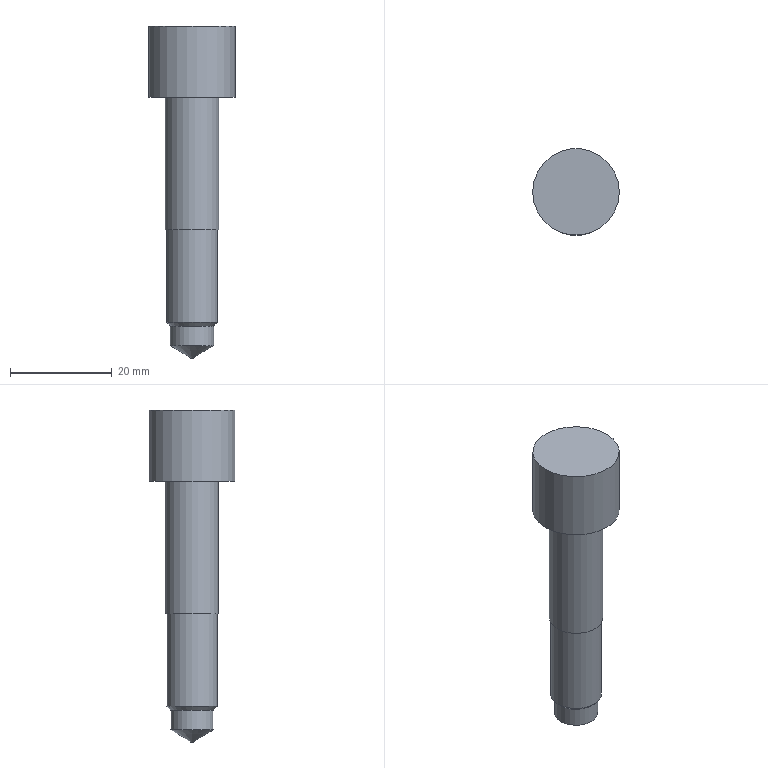Part | NX | features BREP 2 | 2 solids | 21 faces | box 17 x 17 x 65.231 mm | volume 11942 mm3 | plane 14 | cylinder 5 | cone 2 | commonest cylinder face diameters 8.5 x1 10 x1 10.5 x1 16 x1 17 x1
STEP:
#1=CARTESIAN_POINT('',(-4.25,0.,-40.));
#2=VERTEX_POINT('',#1);
#3=CARTESIAN_POINT('',(0.,0.,-40.));
#4=DIRECTION('',(0.,0.,1.));
#5=DIRECTION('',(-1.,0.,0.));
#6=AXIS2_PLACEMENT_3D('',#3,#4,#5);
#7=CIRCLE('',#6,4.25);
#8=EDGE_CURVE('',#2,#2,#7,.T.);
#9=ORIENTED_EDGE('',*,*,#8,.F.);
#10=EDGE_LOOP('',(#9));
#11=FACE_BOUND('',#10,.T.);
#12=CARTESIAN_POINT('',(-4.25,0.,-62.8));
#13=VERTEX_POINT('',#12);
#14=CARTESIAN_POINT('',(0.,0.,-62.8));
#15=DIRECTION('',(0.,0.,-1.));
#16=DIRECTION('',(-1.,0.,0.));
#17=AXIS2_PLACEMENT_3D('',#14,#15,#16);
#18=CIRCLE('',#17,4.25);
#19=EDGE_CURVE('',#13,#13,#18,.T.);
#20=ORIENTED_EDGE('',*,*,#19,.F.);
#21=EDGE_LOOP('',(#20));
#22=FACE_BOUND('',#21,.T.);
#23=CARTESIAN_POINT('',(0.,0.,-62.8));
#24=DIRECTION('',(0.,0.,1.));
#25=DIRECTION('',(-1.,0.,0.));
#26=AXIS2_PLACEMENT_3D('',#23,#24,#25);
#27=CYLINDRICAL_SURFACE('',#26,4.25);
#28=ADVANCED_FACE('',(#11,#22),#27,.T.);
#29=CARTESIAN_POINT('',(-0.2034,0.,-65.231));
#30=VERTEX_POINT('',#29);
#31=CARTESIAN_POINT('',(0.,0.,-65.231));
#32=DIRECTION('',(0.,0.,-1.));
#33=DIRECTION('',(-1.,0.,0.));
#34=AXIS2_PLACEMENT_3D('',#31,#32,#33);
#35=CIRCLE('',#34,0.2034);
#36=EDGE_CURVE('',#30,#30,#35,.T.);
#37=ORIENTED_EDGE('',*,*,#36,.T.);
#38=EDGE_LOOP('',(#37));
#39=FACE_BOUND('',#38,.T.);
#40=CARTESIAN_POINT('',(0.,0.,-65.231));
#41=DIRECTION('',(0.,0.,-1.));
#42=DIRECTION('',(1.,0.,0.));
#43=AXIS2_PLACEMENT_3D('',#40,#41,#42);
#44=PLANE('',#43);
#45=ADVANCED_FACE('',(#39),#44,.T.);
#46=ORIENTED_EDGE('',*,*,#36,.F.);
#47=EDGE_LOOP('',(#46));
#48=FACE_BOUND('',#47,.T.);
#49=ORIENTED_EDGE('',*,*,#19,.T.);
#50=EDGE_LOOP('',(#49));
#51=FACE_BOUND('',#50,.T.);
#52=CARTESIAN_POINT('',(0.,0.,-62.8));
#53=DIRECTION('',(0.,0.,1.));
#54=DIRECTION('',(-1.,0.,0.));
#55=AXIS2_PLACEMENT_3D('',#52,#53,#54);
#56=CONICAL_SURFACE('',#55,4.25,1.03);
#57=ADVANCED_FACE('',(#48,#51),#56,.T.);
#58=ORIENTED_EDGE('',*,*,#8,.T.);
#59=EDGE_LOOP('',(#58));
#60=FACE_BOUND('',#59,.T.);
#61=CARTESIAN_POINT('',(-5.25,0.,-40.));
#62=VERTEX_POINT('',#61);
#63=CARTESIAN_POINT('',(0.,0.,-40.));
#64=DIRECTION('',(0.,0.,-1.));
#65=DIRECTION('',(-1.,0.,0.));
#66=AXIS2_PLACEMENT_3D('',#63,#64,#65);
#67=CIRCLE('',#66,5.25);
#68=EDGE_CURVE('',#62,#62,#67,.T.);
#69=ORIENTED_EDGE('',*,*,#68,.T.);
#70=EDGE_LOOP('',(#69));
#71=FACE_BOUND('',#70,.T.);
#72=CARTESIAN_POINT('',(0.,0.,-40.));
#73=DIRECTION('',(0.,0.,-1.));
#74=DIRECTION('',(1.,0.,0.));
#75=AXIS2_PLACEMENT_3D('',#72,#73,#74);
#76=PLANE('',#75);
#77=ADVANCED_FACE('',(#60,#71),#76,.T.);
#78=ORIENTED_EDGE('',*,*,#68,.F.);
#79=EDGE_LOOP('',(#78));
#80=FACE_BOUND('',#79,.T.);
#81=CARTESIAN_POINT('',(-5.25,0.,-14.));
#82=VERTEX_POINT('',#81);
#83=CARTESIAN_POINT('',(0.,0.,-14.));
#84=DIRECTION('',(0.,0.,-1.));
#85=DIRECTION('',(-1.,0.,0.));
#86=AXIS2_PLACEMENT_3D('',#83,#84,#85);
#87=CIRCLE('',#86,5.25);
#88=EDGE_CURVE('',#82,#82,#87,.T.);
#89=ORIENTED_EDGE('',*,*,#88,.T.);
#90=EDGE_LOOP('',(#89));
#91=FACE_BOUND('',#90,.T.);
#92=CARTESIAN_POINT('',(0.,0.,-14.));
#93=DIRECTION('',(0.,0.,-1.));
#94=DIRECTION('',(1.,0.,0.));
#95=AXIS2_PLACEMENT_3D('',#92,#93,#94);
#96=CYLINDRICAL_SURFACE('',#95,5.25);
#97=ADVANCED_FACE('',(#80,#91),#96,.T.);
#98=CARTESIAN_POINT('',(8.5,0.,0.));
#99=VERTEX_POINT('',#98);
#100=CARTESIAN_POINT('',(0.,0.,0.));
#101=DIRECTION('',(0.,0.,1.));
#102=DIRECTION('',(1.,0.,0.));
#103=AXIS2_PLACEMENT_3D('',#100,#101,#102);
#104=CIRCLE('',#103,8.5);
#105=EDGE_CURVE('',#99,#99,#104,.T.);
#106=ORIENTED_EDGE('',*,*,#105,.T.);
#107=EDGE_LOOP('',(#106));
#108=FACE_BOUND('',#107,.T.);
#109=CARTESIAN_POINT('',(0.,0.,0.));
#110=DIRECTION('',(0.,0.,1.));
#111=DIRECTION('',(-1.,0.,0.));
#112=AXIS2_PLACEMENT_3D('',#109,#110,#111);
#113=PLANE('',#112);
#114=ADVANCED_FACE('',(#108),#113,.T.);
#115=ORIENTED_EDGE('',*,*,#105,.F.);
#116=EDGE_LOOP('',(#115));
#117=FACE_BOUND('',#116,.T.);
#118=CARTESIAN_POINT('',(8.5,0.,-14.));
#119=VERTEX_POINT('',#118);
#120=CARTESIAN_POINT('',(0.,0.,-14.));
#121=DIRECTION('',(0.,0.,1.));
#122=DIRECTION('',(1.,0.,0.));
#123=AXIS2_PLACEMENT_3D('',#120,#121,#122);
#124=CIRCLE('',#123,8.5);
#125=EDGE_CURVE('',#119,#119,#124,.T.);
#126=ORIENTED_EDGE('',*,*,#125,.T.);
#127=EDGE_LOOP('',(#126));
#128=FACE_BOUND('',#127,.T.);
#129=CARTESIAN_POINT('',(0.,0.,-14.));
#130=DIRECTION('',(0.,0.,1.));
#131=DIRECTION('',(-1.,0.,0.));
#132=AXIS2_PLACEMENT_3D('',#129,#130,#131);
#133=CYLINDRICAL_SURFACE('',#132,8.5);
#134=ADVANCED_FACE('',(#117,#128),#133,.T.);
#135=ORIENTED_EDGE('',*,*,#88,.F.);
#136=EDGE_LOOP('',(#135));
#137=FACE_BOUND('',#136,.T.);
#138=ORIENTED_EDGE('',*,*,#125,.F.);
#139=EDGE_LOOP('',(#138));
#140=FACE_BOUND('',#139,.T.);
#141=CARTESIAN_POINT('',(0.,0.,-14.));
#142=DIRECTION('',(0.,0.,-1.));
#143=DIRECTION('',(1.,0.,0.));
#144=AXIS2_PLACEMENT_3D('',#141,#142,#143);
#145=PLANE('',#144);
#146=ADVANCED_FACE('',(#137,#140),#145,.T.);
#147=CLOSED_SHELL('',(#28,#45,#57,#77,#97,#114,#134,#146));
#148=MANIFOLD_SOLID_BREP('',#147);
#149=CARTESIAN_POINT('',(8.,0.,-4.));
#150=VERTEX_POINT('',#149);
#151=CARTESIAN_POINT('',(0.,0.,-4.));
#152=DIRECTION('',(0.,0.,1.));
#153=DIRECTION('',(1.,0.,0.));
#154=AXIS2_PLACEMENT_3D('',#151,#152,#153);
#155=CIRCLE('',#154,8.);
#156=EDGE_CURVE('',#150,#150,#155,.T.);
#157=ORIENTED_EDGE('',*,*,#156,.T.);
#158=EDGE_LOOP('',(#157));
#159=FACE_BOUND('',#158,.T.);
#160=CARTESIAN_POINT('',(4.619,0.,-4.));
#161=VERTEX_POINT('',#160);
#162=CARTESIAN_POINT('',(2.309,-4.,-4.));
#163=VERTEX_POINT('',#162);
#164=CARTESIAN_POINT('',(4.619,0.,-4.));
#165=DIRECTION('',(-0.5,-0.866,0.));
#166=VECTOR('',#165,1000.);
#167=LINE('',#164,#166);
#168=EDGE_CURVE('',#161,#163,#167,.T.);
#169=ORIENTED_EDGE('',*,*,#168,.T.);
#170=CARTESIAN_POINT('',(-2.309,-4.,-4.));
#171=VERTEX_POINT('',#170);
#172=CARTESIAN_POINT('',(2.309,-4.,-4.));
#173=DIRECTION('',(-1.,0.,0.));
#174=VECTOR('',#173,1000.);
#175=LINE('',#172,#174);
#176=EDGE_CURVE('',#163,#171,#175,.T.);
#177=ORIENTED_EDGE('',*,*,#176,.T.);
#178=CARTESIAN_POINT('',(-4.619,0.,-4.));
#179=VERTEX_POINT('',#178);
#180=CARTESIAN_POINT('',(-2.309,-4.,-4.));
#181=DIRECTION('',(-0.5,0.866,0.));
#182=VECTOR('',#181,1000.);
#183=LINE('',#180,#182);
#184=EDGE_CURVE('',#171,#179,#183,.T.);
#185=ORIENTED_EDGE('',*,*,#184,.T.);
#186=CARTESIAN_POINT('',(-2.309,4.,-4.));
#187=VERTEX_POINT('',#186);
#188=CARTESIAN_POINT('',(-4.619,0.,-4.));
#189=DIRECTION('',(0.5,0.866,0.));
#190=VECTOR('',#189,1000.);
#191=LINE('',#188,#190);
#192=EDGE_CURVE('',#179,#187,#191,.T.);
#193=ORIENTED_EDGE('',*,*,#192,.T.);
#194=CARTESIAN_POINT('',(2.309,4.,-4.));
#195=VERTEX_POINT('',#194);
#196=CARTESIAN_POINT('',(-2.309,4.,-4.));
#197=DIRECTION('',(1.,0.,0.));
#198=VECTOR('',#197,1000.);
#199=LINE('',#196,#198);
#200=EDGE_CURVE('',#187,#195,#199,.T.);
#201=ORIENTED_EDGE('',*,*,#200,.T.);
#202=CARTESIAN_POINT('',(2.309,4.,-4.));
#203=DIRECTION('',(0.5,-0.866,0.));
#204=VECTOR('',#203,1000.);
#205=LINE('',#202,#204);
#206=EDGE_CURVE('',#195,#161,#205,.T.);
#207=ORIENTED_EDGE('',*,*,#206,.T.);
#208=EDGE_LOOP('',(#169,#177,#185,#193,#201,#207));
#209=FACE_BOUND('',#208,.T.);
#210=CARTESIAN_POINT('',(0.,0.,-4.));
#211=DIRECTION('',(0.,0.,1.));
#212=DIRECTION('',(-1.,0.,0.));
#213=AXIS2_PLACEMENT_3D('',#210,#211,#212);
#214=PLANE('',#213);
#215=ADVANCED_FACE('',(#159,#209),#214,.T.);
#216=CARTESIAN_POINT('',(5.,0.,-58.25));
#217=VERTEX_POINT('',#216);
#218=CARTESIAN_POINT('',(0.,0.,-58.25));
#219=DIRECTION('',(0.,0.,1.));
#220=DIRECTION('',(1.,0.,0.));
#221=AXIS2_PLACEMENT_3D('',#218,#219,#220);
#222=CIRCLE('',#221,5.);
#223=EDGE_CURVE('',#217,#217,#222,.T.);
#224=ORIENTED_EDGE('',*,*,#223,.T.);
#225=EDGE_LOOP('',(#224));
#226=FACE_BOUND('',#225,.T.);
#227=CARTESIAN_POINT('',(5.,0.,-14.));
#228=VERTEX_POINT('',#227);
#229=CARTESIAN_POINT('',(0.,0.,-14.));
#230=DIRECTION('',(0.,0.,1.));
#231=DIRECTION('',(1.,0.,0.));
#232=AXIS2_PLACEMENT_3D('',#229,#230,#231);
#233=CIRCLE('',#232,5.);
#234=EDGE_CURVE('',#228,#228,#233,.T.);
#235=ORIENTED_EDGE('',*,*,#234,.F.);
#236=EDGE_LOOP('',(#235));
#237=FACE_BOUND('',#236,.T.);
#238=CARTESIAN_POINT('',(0.,0.,-59.));
#239=DIRECTION('',(0.,0.,1.));
#240=DIRECTION('',(-1.,0.,0.));
#241=AXIS2_PLACEMENT_3D('',#238,#239,#240);
#242=CYLINDRICAL_SURFACE('',#241,5.);
#243=ADVANCED_FACE('',(#226,#237),#242,.T.);
#244=CARTESIAN_POINT('',(4.25,0.,-59.));
#245=VERTEX_POINT('',#244);
#246=CARTESIAN_POINT('',(0.,0.,-59.));
#247=DIRECTION('',(0.,0.,-1.));
#248=DIRECTION('',(1.,0.,0.));
#249=AXIS2_PLACEMENT_3D('',#246,#247,#248);
#250=CIRCLE('',#249,4.25);
#251=EDGE_CURVE('',#245,#245,#250,.T.);
#252=ORIENTED_EDGE('',*,*,#251,.T.);
#253=EDGE_LOOP('',(#252));
#254=FACE_BOUND('',#253,.T.);
#255=CARTESIAN_POINT('',(0.,0.,-59.));
#256=DIRECTION('',(0.,0.,1.));
#257=DIRECTION('',(-1.,0.,0.));
#258=AXIS2_PLACEMENT_3D('',#255,#256,#257);
#259=PLANE('',#258);
#260=ADVANCED_FACE('',(#254),#259,.F.);
#261=ORIENTED_EDGE('',*,*,#234,.T.);
#262=EDGE_LOOP('',(#261));
#263=FACE_BOUND('',#262,.T.);
#264=CARTESIAN_POINT('',(8.,0.,-14.));
#265=VERTEX_POINT('',#264);
#266=CARTESIAN_POINT('',(0.,0.,-14.));
#267=DIRECTION('',(0.,0.,1.));
#268=DIRECTION('',(1.,0.,0.));
#269=AXIS2_PLACEMENT_3D('',#266,#267,#268);
#270=CIRCLE('',#269,8.);
#271=EDGE_CURVE('',#265,#265,#270,.T.);
#272=ORIENTED_EDGE('',*,*,#271,.F.);
#273=EDGE_LOOP('',(#272));
#274=FACE_BOUND('',#273,.T.);
#275=CARTESIAN_POINT('',(0.,0.,-14.));
#276=DIRECTION('',(0.,0.,-1.));
#277=DIRECTION('',(1.,0.,0.));
#278=AXIS2_PLACEMENT_3D('',#275,#276,#277);
#279=PLANE('',#278);
#280=ADVANCED_FACE('',(#263,#274),#279,.T.);
#281=ORIENTED_EDGE('',*,*,#156,.F.);
#282=EDGE_LOOP('',(#281));
#283=FACE_BOUND('',#282,.T.);
#284=ORIENTED_EDGE('',*,*,#271,.T.);
#285=EDGE_LOOP('',(#284));
#286=FACE_BOUND('',#285,.T.);
#287=CARTESIAN_POINT('',(0.,0.,-14.));
#288=DIRECTION('',(0.,0.,1.));
#289=DIRECTION('',(-1.,0.,0.));
#290=AXIS2_PLACEMENT_3D('',#287,#288,#289);
#291=CYLINDRICAL_SURFACE('',#290,8.);
#292=ADVANCED_FACE('',(#283,#286),#291,.T.);
#293=ORIENTED_EDGE('',*,*,#251,.F.);
#294=EDGE_LOOP('',(#293));
#295=FACE_BOUND('',#294,.T.);
#296=ORIENTED_EDGE('',*,*,#223,.F.);
#297=EDGE_LOOP('',(#296));
#298=FACE_BOUND('',#297,.T.);
#299=CARTESIAN_POINT('',(0.,0.,-58.25));
#300=DIRECTION('',(0.,0.,1.));
#301=DIRECTION('',(-1.,0.,0.));
#302=AXIS2_PLACEMENT_3D('',#299,#300,#301);
#303=CONICAL_SURFACE('',#302,5.,0.7854);
#304=ADVANCED_FACE('',(#295,#298),#303,.T.);
#305=ORIENTED_EDGE('',*,*,#176,.F.);
#306=CARTESIAN_POINT('',(2.309,-4.,-10.6));
#307=VERTEX_POINT('',#306);
#308=CARTESIAN_POINT('',(2.309,-4.,-10.6));
#309=DIRECTION('',(0.,0.,1.));
#310=VECTOR('',#309,1000.);
#311=LINE('',#308,#310);
#312=EDGE_CURVE('',#307,#163,#311,.T.);
#313=ORIENTED_EDGE('',*,*,#312,.F.);
#314=CARTESIAN_POINT('',(-2.309,-4.,-10.6));
#315=VERTEX_POINT('',#314);
#316=CARTESIAN_POINT('',(2.309,-4.,-10.6));
#317=DIRECTION('',(-1.,0.,0.));
#318=VECTOR('',#317,1000.);
#319=LINE('',#316,#318);
#320=EDGE_CURVE('',#307,#315,#319,.T.);
#321=ORIENTED_EDGE('',*,*,#320,.T.);
#322=CARTESIAN_POINT('',(-2.309,-4.,-10.6));
#323=DIRECTION('',(0.,0.,1.));
#324=VECTOR('',#323,1000.);
#325=LINE('',#322,#324);
#326=EDGE_CURVE('',#315,#171,#325,.T.);
#327=ORIENTED_EDGE('',*,*,#326,.T.);
#328=EDGE_LOOP('',(#305,#313,#321,#327));
#329=FACE_BOUND('',#328,.T.);
#330=CARTESIAN_POINT('',(2.309,-4.,-10.6));
#331=DIRECTION('',(0.,1.,0.));
#332=DIRECTION('',(0.,0.,-1.));
#333=AXIS2_PLACEMENT_3D('',#330,#331,#332);
#334=PLANE('',#333);
#335=ADVANCED_FACE('',(#329),#334,.T.);
#336=ORIENTED_EDGE('',*,*,#184,.F.);
#337=ORIENTED_EDGE('',*,*,#326,.F.);
#338=CARTESIAN_POINT('',(-4.619,0.,-10.6));
#339=VERTEX_POINT('',#338);
#340=CARTESIAN_POINT('',(-2.309,-4.,-10.6));
#341=DIRECTION('',(-0.5,0.866,0.));
#342=VECTOR('',#341,1000.);
#343=LINE('',#340,#342);
#344=EDGE_CURVE('',#315,#339,#343,.T.);
#345=ORIENTED_EDGE('',*,*,#344,.T.);
#346=CARTESIAN_POINT('',(-4.619,0.,-10.6));
#347=DIRECTION('',(0.,0.,1.));
#348=VECTOR('',#347,1000.);
#349=LINE('',#346,#348);
#350=EDGE_CURVE('',#339,#179,#349,.T.);
#351=ORIENTED_EDGE('',*,*,#350,.T.);
#352=EDGE_LOOP('',(#336,#337,#345,#351));
#353=FACE_BOUND('',#352,.T.);
#354=CARTESIAN_POINT('',(-2.309,-4.,-10.6));
#355=DIRECTION('',(0.866,0.5,0.));
#356=DIRECTION('',(0.5,-0.866,0.));
#357=AXIS2_PLACEMENT_3D('',#354,#355,#356);
#358=PLANE('',#357);
#359=ADVANCED_FACE('',(#353),#358,.T.);
#360=ORIENTED_EDGE('',*,*,#192,.F.);
#361=ORIENTED_EDGE('',*,*,#350,.F.);
#362=CARTESIAN_POINT('',(-2.309,4.,-10.6));
#363=VERTEX_POINT('',#362);
#364=CARTESIAN_POINT('',(-4.619,0.,-10.6));
#365=DIRECTION('',(0.5,0.866,0.));
#366=VECTOR('',#365,1000.);
#367=LINE('',#364,#366);
#368=EDGE_CURVE('',#339,#363,#367,.T.);
#369=ORIENTED_EDGE('',*,*,#368,.T.);
#370=CARTESIAN_POINT('',(-2.309,4.,-10.6));
#371=DIRECTION('',(0.,0.,1.));
#372=VECTOR('',#371,1000.);
#373=LINE('',#370,#372);
#374=EDGE_CURVE('',#363,#187,#373,.T.);
#375=ORIENTED_EDGE('',*,*,#374,.T.);
#376=EDGE_LOOP('',(#360,#361,#369,#375));
#377=FACE_BOUND('',#376,.T.);
#378=CARTESIAN_POINT('',(-4.619,0.,-10.6));
#379=DIRECTION('',(0.866,-0.5,0.));
#380=DIRECTION('',(-0.5,-0.866,0.));
#381=AXIS2_PLACEMENT_3D('',#378,#379,#380);
#382=PLANE('',#381);
#383=ADVANCED_FACE('',(#377),#382,.T.);
#384=ORIENTED_EDGE('',*,*,#200,.F.);
#385=ORIENTED_EDGE('',*,*,#374,.F.);
#386=CARTESIAN_POINT('',(2.309,4.,-10.6));
#387=VERTEX_POINT('',#386);
#388=CARTESIAN_POINT('',(-2.309,4.,-10.6));
#389=DIRECTION('',(1.,0.,0.));
#390=VECTOR('',#389,1000.);
#391=LINE('',#388,#390);
#392=EDGE_CURVE('',#363,#387,#391,.T.);
#393=ORIENTED_EDGE('',*,*,#392,.T.);
#394=CARTESIAN_POINT('',(2.309,4.,-10.6));
#395=DIRECTION('',(0.,0.,1.));
#396=VECTOR('',#395,1000.);
#397=LINE('',#394,#396);
#398=EDGE_CURVE('',#387,#195,#397,.T.);
#399=ORIENTED_EDGE('',*,*,#398,.T.);
#400=EDGE_LOOP('',(#384,#385,#393,#399));
#401=FACE_BOUND('',#400,.T.);
#402=CARTESIAN_POINT('',(-2.309,4.,-10.6));
#403=DIRECTION('',(0.,-1.,0.));
#404=DIRECTION('',(0.,0.,1.));
#405=AXIS2_PLACEMENT_3D('',#402,#403,#404);
#406=PLANE('',#405);
#407=ADVANCED_FACE('',(#401),#406,.T.);
#408=ORIENTED_EDGE('',*,*,#206,.F.);
#409=ORIENTED_EDGE('',*,*,#398,.F.);
#410=CARTESIAN_POINT('',(4.619,0.,-10.6));
#411=VERTEX_POINT('',#410);
#412=CARTESIAN_POINT('',(2.309,4.,-10.6));
#413=DIRECTION('',(0.5,-0.866,0.));
#414=VECTOR('',#413,1000.);
#415=LINE('',#412,#414);
#416=EDGE_CURVE('',#387,#411,#415,.T.);
#417=ORIENTED_EDGE('',*,*,#416,.T.);
#418=CARTESIAN_POINT('',(4.619,0.,-10.6));
#419=DIRECTION('',(0.,0.,1.));
#420=VECTOR('',#419,1000.);
#421=LINE('',#418,#420);
#422=EDGE_CURVE('',#411,#161,#421,.T.);
#423=ORIENTED_EDGE('',*,*,#422,.T.);
#424=EDGE_LOOP('',(#408,#409,#417,#423));
#425=FACE_BOUND('',#424,.T.);
#426=CARTESIAN_POINT('',(2.309,4.,-10.6));
#427=DIRECTION('',(-0.866,-0.5,0.));
#428=DIRECTION('',(-0.5,0.866,0.));
#429=AXIS2_PLACEMENT_3D('',#426,#427,#428);
#430=PLANE('',#429);
#431=ADVANCED_FACE('',(#425),#430,.T.);
#432=ORIENTED_EDGE('',*,*,#168,.F.);
#433=ORIENTED_EDGE('',*,*,#422,.F.);
#434=CARTESIAN_POINT('',(4.619,0.,-10.6));
#435=DIRECTION('',(-0.5,-0.866,0.));
#436=VECTOR('',#435,1000.);
#437=LINE('',#434,#436);
#438=EDGE_CURVE('',#411,#307,#437,.T.);
#439=ORIENTED_EDGE('',*,*,#438,.T.);
#440=ORIENTED_EDGE('',*,*,#312,.T.);
#441=EDGE_LOOP('',(#432,#433,#439,#440));
#442=FACE_BOUND('',#441,.T.);
#443=CARTESIAN_POINT('',(4.619,0.,-10.6));
#444=DIRECTION('',(-0.866,0.5,0.));
#445=DIRECTION('',(0.5,0.866,0.));
#446=AXIS2_PLACEMENT_3D('',#443,#444,#445);
#447=PLANE('',#446);
#448=ADVANCED_FACE('',(#442),#447,.T.);
#449=ORIENTED_EDGE('',*,*,#320,.F.);
#450=ORIENTED_EDGE('',*,*,#438,.F.);
#451=ORIENTED_EDGE('',*,*,#416,.F.);
#452=ORIENTED_EDGE('',*,*,#392,.F.);
#453=ORIENTED_EDGE('',*,*,#368,.F.);
#454=ORIENTED_EDGE('',*,*,#344,.F.);
#455=EDGE_LOOP('',(#449,#450,#451,#452,#453,#454));
#456=FACE_BOUND('',#455,.T.);
#457=CARTESIAN_POINT('',(-6.928,-4.,-10.6));
#458=DIRECTION('',(0.,0.,-1.));
#459=DIRECTION('',(1.,0.,0.));
#460=AXIS2_PLACEMENT_3D('',#457,#458,#459);
#461=PLANE('',#460);
#462=ADVANCED_FACE('',(#456),#461,.F.);
#463=CLOSED_SHELL('',(#215,#243,#260,#280,#292,#304,#335,#359,#383,#407,#431,#448,#462));
#464=MANIFOLD_SOLID_BREP('',#463);
#465=(LENGTH_UNIT()NAMED_UNIT(*)SI_UNIT(.MILLI.,.METRE.));
#466=UNCERTAINTY_MEASURE_WITH_UNIT(LENGTH_MEASURE(0.00001),#465,'','');
#467=(NAMED_UNIT(*)PLANE_ANGLE_UNIT()SI_UNIT($,.RADIAN.));
#468=(NAMED_UNIT(*)SI_UNIT($,.STERADIAN.)SOLID_ANGLE_UNIT());
#469=(GEOMETRIC_REPRESENTATION_CONTEXT(3)GLOBAL_UNCERTAINTY_ASSIGNED_CONTEXT((#466))GLOBAL_UNIT_ASSIGNED_CONTEXT((#465,#467,#468))REPRESENTATION_CONTEXT('',''));
#470=ADVANCED_BREP_SHAPE_REPRESENTATION('',(#148,#464),#469);